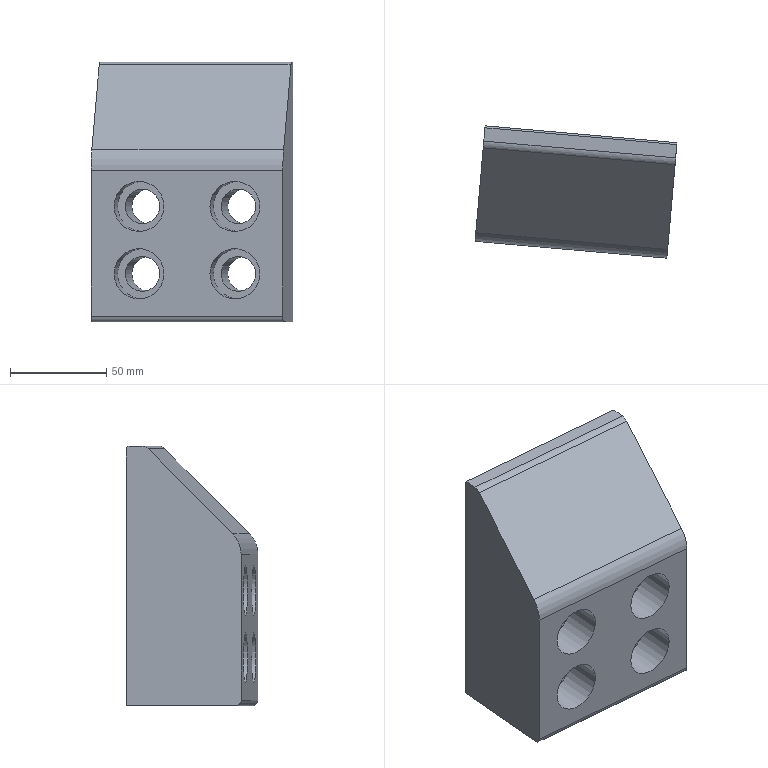Part | NX | features solid 2 | 1 solid | 23 faces | box 104.849 x 68.487 x 135 mm | volume 601030 mm3 | plane 12 | cylinder 11 | commonest cylinder face diameters 18 x4 26 x4 6 x1 10 x1 30 x1
STEP:
#1=CARTESIAN_POINT('',(231.007,-228.001,-65.));
#2=VERTEX_POINT('',#1);
#3=CARTESIAN_POINT('',(235.975,-171.218,-65.));
#4=VERTEX_POINT('',#3);
#5=CARTESIAN_POINT('',(229.874,-240.952,-65.));
#6=DIRECTION('',(0.08716,0.9962,0.));
#7=VECTOR('',#6,1000.);
#8=LINE('',#5,#7);
#9=EDGE_CURVE('',#2,#4,#8,.T.);
#10=ORIENTED_EDGE('',*,*,#9,.F.);
#11=CARTESIAN_POINT('',(230.746,-230.99,-62.));
#12=VERTEX_POINT('',#11);
#13=CARTESIAN_POINT('',(231.007,-228.001,-62.));
#14=DIRECTION('',(0.9962,-0.08716,0.));
#15=DIRECTION('',(0.,0.,1.));
#16=AXIS2_PLACEMENT_3D('',#13,#14,#15);
#17=CIRCLE('',#16,3.);
#18=EDGE_CURVE('',#2,#12,#17,.F.);
#19=ORIENTED_EDGE('',*,*,#18,.T.);
#20=CARTESIAN_POINT('',(230.746,-230.99,13.787));
#21=VERTEX_POINT('',#20);
#22=CARTESIAN_POINT('',(230.746,-230.99,-100.));
#23=DIRECTION('',(0.,0.,-1.));
#24=VECTOR('',#23,1000.);
#25=LINE('',#22,#24);
#26=EDGE_CURVE('',#21,#12,#25,.T.);
#27=ORIENTED_EDGE('',*,*,#26,.F.);
#28=CARTESIAN_POINT('',(231.129,-226.613,24.393));
#29=VERTEX_POINT('',#28);
#30=CARTESIAN_POINT('',(232.053,-216.047,13.787));
#31=DIRECTION('',(0.9962,-0.08716,0.));
#32=DIRECTION('',(0.,0.,1.));
#33=AXIS2_PLACEMENT_3D('',#30,#31,#32);
#34=CIRCLE('',#33,15.);
#35=EDGE_CURVE('',#21,#29,#34,.F.);
#36=ORIENTED_EDGE('',*,*,#35,.T.);
#37=CARTESIAN_POINT('',(234.976,-182.639,68.536));
#38=VERTEX_POINT('',#37);
#39=CARTESIAN_POINT('',(232.489,-211.066,40.));
#40=DIRECTION('',(0.06163,0.7044,0.7071));
#41=VECTOR('',#40,1000.);
#42=LINE('',#39,#41);
#43=EDGE_CURVE('',#29,#38,#42,.T.);
#44=ORIENTED_EDGE('',*,*,#43,.T.);
#45=CARTESIAN_POINT('',(235.284,-179.117,70.));
#46=VERTEX_POINT('',#45);
#47=CARTESIAN_POINT('',(235.284,-179.117,65.));
#48=DIRECTION('',(0.9962,-0.08716,0.));
#49=DIRECTION('',(0.,0.,1.));
#50=AXIS2_PLACEMENT_3D('',#47,#48,#49);
#51=CIRCLE('',#50,5.);
#52=EDGE_CURVE('',#38,#46,#51,.F.);
#53=ORIENTED_EDGE('',*,*,#52,.T.);
#54=CARTESIAN_POINT('',(235.888,-172.214,70.));
#55=VERTEX_POINT('',#54);
#56=CARTESIAN_POINT('',(229.874,-240.952,70.));
#57=DIRECTION('',(0.08716,0.9962,0.));
#58=VECTOR('',#57,1000.);
#59=LINE('',#56,#58);
#60=EDGE_CURVE('',#46,#55,#59,.T.);
#61=ORIENTED_EDGE('',*,*,#60,.T.);
#62=CARTESIAN_POINT('',(235.975,-171.218,69.));
#63=VERTEX_POINT('',#62);
#64=CARTESIAN_POINT('',(235.888,-172.214,70.));
#65=DIRECTION('',(0.06163,0.7044,-0.7071));
#66=VECTOR('',#65,1000.);
#67=LINE('',#64,#66);
#68=EDGE_CURVE('',#55,#63,#67,.T.);
#69=ORIENTED_EDGE('',*,*,#68,.T.);
#70=CARTESIAN_POINT('',(235.975,-171.218,70.));
#71=DIRECTION('',(0.,0.,-1.));
#72=VECTOR('',#71,1000.);
#73=LINE('',#70,#72);
#74=EDGE_CURVE('',#63,#4,#73,.T.);
#75=ORIENTED_EDGE('',*,*,#74,.T.);
#76=EDGE_LOOP('',(#10,#19,#27,#36,#44,#53,#61,#69,#75));
#77=FACE_BOUND('',#76,.T.);
#78=CARTESIAN_POINT('',(229.874,-240.952,70.));
#79=DIRECTION('',(0.9962,-0.08716,0.));
#80=DIRECTION('',(0.,0.,1.));
#81=AXIS2_PLACEMENT_3D('',#78,#79,#80);
#82=PLANE('',#81);
#83=ADVANCED_FACE('',(#77),#82,.F.);
#84=CARTESIAN_POINT('',(330.627,-236.717,-65.));
#85=VERTEX_POINT('',#84);
#86=CARTESIAN_POINT('',(335.595,-179.934,-65.));
#87=VERTEX_POINT('',#86);
#88=CARTESIAN_POINT('',(329.494,-249.667,-65.));
#89=DIRECTION('',(0.08716,0.9962,0.));
#90=VECTOR('',#89,1000.);
#91=LINE('',#88,#90);
#92=EDGE_CURVE('',#85,#87,#91,.T.);
#93=ORIENTED_EDGE('',*,*,#92,.F.);
#94=CARTESIAN_POINT('',(231.007,-228.001,-65.));
#95=DIRECTION('',(-0.9962,0.08716,0.));
#96=VECTOR('',#95,1000.);
#97=LINE('',#94,#96);
#98=EDGE_CURVE('',#85,#2,#97,.T.);
#99=ORIENTED_EDGE('',*,*,#98,.T.);
#100=ORIENTED_EDGE('',*,*,#9,.T.);
#101=CARTESIAN_POINT('',(335.595,-179.934,-65.));
#102=DIRECTION('',(-0.9962,0.08716,0.));
#103=VECTOR('',#102,1000.);
#104=LINE('',#101,#103);
#105=EDGE_CURVE('',#87,#4,#104,.T.);
#106=ORIENTED_EDGE('',*,*,#105,.F.);
#107=EDGE_LOOP('',(#93,#99,#100,#106));
#108=FACE_BOUND('',#107,.T.);
#109=CARTESIAN_POINT('',(329.494,-249.667,-65.));
#110=DIRECTION('',(0.,0.,-1.));
#111=DIRECTION('',(0.08716,0.9962,0.));
#112=AXIS2_PLACEMENT_3D('',#109,#110,#111);
#113=PLANE('',#112);
#114=ADVANCED_FACE('',(#108),#113,.T.);
#115=CARTESIAN_POINT('',(330.365,-239.705,13.787));
#116=VERTEX_POINT('',#115);
#117=CARTESIAN_POINT('',(330.365,-239.705,-62.));
#118=VERTEX_POINT('',#117);
#119=CARTESIAN_POINT('',(330.365,-239.705,-100.));
#120=DIRECTION('',(0.,0.,-1.));
#121=VECTOR('',#120,1000.);
#122=LINE('',#119,#121);
#123=EDGE_CURVE('',#116,#118,#122,.T.);
#124=ORIENTED_EDGE('',*,*,#123,.T.);
#125=CARTESIAN_POINT('',(330.627,-236.717,-62.));
#126=DIRECTION('',(0.9962,-0.08716,0.));
#127=DIRECTION('',(0.,0.,1.));
#128=AXIS2_PLACEMENT_3D('',#125,#126,#127);
#129=CIRCLE('',#128,3.);
#130=EDGE_CURVE('',#118,#85,#129,.T.);
#131=ORIENTED_EDGE('',*,*,#130,.T.);
#132=ORIENTED_EDGE('',*,*,#92,.T.);
#133=CARTESIAN_POINT('',(335.595,-179.934,69.));
#134=VERTEX_POINT('',#133);
#135=CARTESIAN_POINT('',(335.595,-179.934,70.));
#136=DIRECTION('',(0.,0.,-1.));
#137=VECTOR('',#136,1000.);
#138=LINE('',#135,#137);
#139=EDGE_CURVE('',#134,#87,#138,.T.);
#140=ORIENTED_EDGE('',*,*,#139,.F.);
#141=CARTESIAN_POINT('',(335.508,-180.93,70.));
#142=VERTEX_POINT('',#141);
#143=CARTESIAN_POINT('',(332.501,-215.299,104.5));
#144=DIRECTION('',(-0.06163,-0.7044,0.7071));
#145=VECTOR('',#144,1000.);
#146=LINE('',#143,#145);
#147=EDGE_CURVE('',#134,#142,#146,.T.);
#148=ORIENTED_EDGE('',*,*,#147,.T.);
#149=CARTESIAN_POINT('',(334.904,-187.832,70.));
#150=VERTEX_POINT('',#149);
#151=CARTESIAN_POINT('',(329.494,-249.667,70.));
#152=DIRECTION('',(0.08716,0.9962,0.));
#153=VECTOR('',#152,1000.);
#154=LINE('',#151,#153);
#155=EDGE_CURVE('',#150,#142,#154,.T.);
#156=ORIENTED_EDGE('',*,*,#155,.F.);
#157=CARTESIAN_POINT('',(334.596,-191.355,68.536));
#158=VERTEX_POINT('',#157);
#159=CARTESIAN_POINT('',(334.904,-187.832,65.));
#160=DIRECTION('',(0.9962,-0.08716,0.));
#161=DIRECTION('',(0.,0.,1.));
#162=AXIS2_PLACEMENT_3D('',#159,#160,#161);
#163=CIRCLE('',#162,5.);
#164=EDGE_CURVE('',#150,#158,#163,.T.);
#165=ORIENTED_EDGE('',*,*,#164,.T.);
#166=CARTESIAN_POINT('',(330.748,-235.329,24.393));
#167=VERTEX_POINT('',#166);
#168=CARTESIAN_POINT('',(332.109,-219.782,40.));
#169=DIRECTION('',(0.06163,0.7044,0.7071));
#170=VECTOR('',#169,1000.);
#171=LINE('',#168,#170);
#172=EDGE_CURVE('',#167,#158,#171,.T.);
#173=ORIENTED_EDGE('',*,*,#172,.F.);
#174=CARTESIAN_POINT('',(331.673,-224.762,13.787));
#175=DIRECTION('',(0.9962,-0.08716,0.));
#176=DIRECTION('',(0.,0.,1.));
#177=AXIS2_PLACEMENT_3D('',#174,#175,#176);
#178=CIRCLE('',#177,15.);
#179=EDGE_CURVE('',#167,#116,#178,.T.);
#180=ORIENTED_EDGE('',*,*,#179,.T.);
#181=EDGE_LOOP('',(#124,#131,#132,#140,#148,#156,#165,#173,#180));
#182=FACE_BOUND('',#181,.T.);
#183=CARTESIAN_POINT('',(329.494,-249.667,70.));
#184=DIRECTION('',(0.9962,-0.08716,0.));
#185=DIRECTION('',(0.,0.,1.));
#186=AXIS2_PLACEMENT_3D('',#183,#184,#185);
#187=PLANE('',#186);
#188=ADVANCED_FACE('',(#182),#187,.T.);
#189=ORIENTED_EDGE('',*,*,#155,.T.);
#190=CARTESIAN_POINT('',(235.888,-172.214,70.));
#191=DIRECTION('',(-0.9962,0.08716,0.));
#192=VECTOR('',#191,1000.);
#193=LINE('',#190,#192);
#194=EDGE_CURVE('',#142,#55,#193,.T.);
#195=ORIENTED_EDGE('',*,*,#194,.T.);
#196=ORIENTED_EDGE('',*,*,#60,.F.);
#197=CARTESIAN_POINT('',(334.904,-187.832,70.));
#198=DIRECTION('',(0.9962,-0.08716,0.));
#199=VECTOR('',#198,1000.);
#200=LINE('',#197,#199);
#201=EDGE_CURVE('',#46,#150,#200,.T.);
#202=ORIENTED_EDGE('',*,*,#201,.T.);
#203=EDGE_LOOP('',(#189,#195,#196,#202));
#204=FACE_BOUND('',#203,.T.);
#205=CARTESIAN_POINT('',(329.494,-249.667,70.));
#206=DIRECTION('',(0.,0.,-1.));
#207=DIRECTION('',(0.08716,0.9962,0.));
#208=AXIS2_PLACEMENT_3D('',#205,#206,#207);
#209=PLANE('',#208);
#210=ADVANCED_FACE('',(#204),#209,.F.);
#211=CARTESIAN_POINT('',(242.7,-232.036,-40.));
#212=VERTEX_POINT('',#211);
#213=CARTESIAN_POINT('',(255.651,-233.169,-40.));
#214=DIRECTION('',(0.08716,0.9962,0.));
#215=DIRECTION('',(-0.9962,0.08716,0.));
#216=AXIS2_PLACEMENT_3D('',#213,#214,#215);
#217=CIRCLE('',#216,13.);
#218=EDGE_CURVE('',#212,#212,#217,.T.);
#219=ORIENTED_EDGE('',*,*,#218,.T.);
#220=EDGE_LOOP('',(#219));
#221=FACE_BOUND('',#220,.T.);
#222=CARTESIAN_POINT('',(292.51,-236.393,-40.));
#223=VERTEX_POINT('',#222);
#224=CARTESIAN_POINT('',(305.461,-237.527,-40.));
#225=DIRECTION('',(0.08716,0.9962,0.));
#226=DIRECTION('',(-0.9962,0.08716,0.));
#227=AXIS2_PLACEMENT_3D('',#224,#225,#226);
#228=CIRCLE('',#227,13.);
#229=EDGE_CURVE('',#223,#223,#228,.T.);
#230=ORIENTED_EDGE('',*,*,#229,.T.);
#231=EDGE_LOOP('',(#230));
#232=FACE_BOUND('',#231,.T.);
#233=CARTESIAN_POINT('',(292.51,-236.393,-5.));
#234=VERTEX_POINT('',#233);
#235=CARTESIAN_POINT('',(305.461,-237.527,-5.));
#236=DIRECTION('',(0.08716,0.9962,0.));
#237=DIRECTION('',(-0.9962,0.08716,0.));
#238=AXIS2_PLACEMENT_3D('',#235,#236,#237);
#239=CIRCLE('',#238,13.);
#240=EDGE_CURVE('',#234,#234,#239,.T.);
#241=ORIENTED_EDGE('',*,*,#240,.T.);
#242=EDGE_LOOP('',(#241));
#243=FACE_BOUND('',#242,.T.);
#244=CARTESIAN_POINT('',(242.7,-232.036,-5.));
#245=VERTEX_POINT('',#244);
#246=CARTESIAN_POINT('',(255.651,-233.169,-5.));
#247=DIRECTION('',(0.08716,0.9962,0.));
#248=DIRECTION('',(-0.9962,0.08716,0.));
#249=AXIS2_PLACEMENT_3D('',#246,#247,#248);
#250=CIRCLE('',#249,13.);
#251=EDGE_CURVE('',#245,#245,#250,.T.);
#252=ORIENTED_EDGE('',*,*,#251,.T.);
#253=EDGE_LOOP('',(#252));
#254=FACE_BOUND('',#253,.T.);
#255=ORIENTED_EDGE('',*,*,#26,.T.);
#256=CARTESIAN_POINT('',(330.365,-239.705,-62.));
#257=DIRECTION('',(-0.9962,0.08716,0.));
#258=VECTOR('',#257,1000.);
#259=LINE('',#256,#258);
#260=EDGE_CURVE('',#12,#118,#259,.F.);
#261=ORIENTED_EDGE('',*,*,#260,.T.);
#262=ORIENTED_EDGE('',*,*,#123,.F.);
#263=CARTESIAN_POINT('',(230.746,-230.99,13.787));
#264=DIRECTION('',(-0.9962,0.08716,0.));
#265=VECTOR('',#264,1000.);
#266=LINE('',#263,#265);
#267=EDGE_CURVE('',#116,#21,#266,.T.);
#268=ORIENTED_EDGE('',*,*,#267,.T.);
#269=EDGE_LOOP('',(#255,#261,#262,#268));
#270=FACE_BOUND('',#269,.T.);
#271=CARTESIAN_POINT('',(230.746,-230.99,-100.));
#272=DIRECTION('',(0.08716,0.9962,0.));
#273=DIRECTION('',(-0.9962,0.08716,0.));
#274=AXIS2_PLACEMENT_3D('',#271,#272,#273);
#275=PLANE('',#274);
#276=ADVANCED_FACE('',(#221,#232,#243,#254,#270),#275,.F.);
#277=CARTESIAN_POINT('',(251.914,-172.613,-40.));
#278=VERTEX_POINT('',#277);
#279=CARTESIAN_POINT('',(260.88,-173.397,-40.));
#280=DIRECTION('',(0.08716,0.9962,0.));
#281=DIRECTION('',(-0.9962,0.08716,0.));
#282=AXIS2_PLACEMENT_3D('',#279,#280,#281);
#283=CIRCLE('',#282,9.);
#284=EDGE_CURVE('',#278,#278,#283,.T.);
#285=ORIENTED_EDGE('',*,*,#284,.F.);
#286=EDGE_LOOP('',(#285));
#287=FACE_BOUND('',#286,.T.);
#288=CARTESIAN_POINT('',(301.724,-176.97,-40.));
#289=VERTEX_POINT('',#288);
#290=CARTESIAN_POINT('',(310.69,-177.755,-40.));
#291=DIRECTION('',(0.08716,0.9962,0.));
#292=DIRECTION('',(-0.9962,0.08716,0.));
#293=AXIS2_PLACEMENT_3D('',#290,#291,#292);
#294=CIRCLE('',#293,9.);
#295=EDGE_CURVE('',#289,#289,#294,.T.);
#296=ORIENTED_EDGE('',*,*,#295,.F.);
#297=EDGE_LOOP('',(#296));
#298=FACE_BOUND('',#297,.T.);
#299=CARTESIAN_POINT('',(301.724,-176.97,-5.));
#300=VERTEX_POINT('',#299);
#301=CARTESIAN_POINT('',(310.69,-177.755,-5.));
#302=DIRECTION('',(0.08716,0.9962,0.));
#303=DIRECTION('',(-0.9962,0.08716,0.));
#304=AXIS2_PLACEMENT_3D('',#301,#302,#303);
#305=CIRCLE('',#304,9.);
#306=EDGE_CURVE('',#300,#300,#305,.T.);
#307=ORIENTED_EDGE('',*,*,#306,.F.);
#308=EDGE_LOOP('',(#307));
#309=FACE_BOUND('',#308,.T.);
#310=CARTESIAN_POINT('',(251.914,-172.613,-5.));
#311=VERTEX_POINT('',#310);
#312=CARTESIAN_POINT('',(260.88,-173.397,-5.));
#313=DIRECTION('',(0.08716,0.9962,0.));
#314=DIRECTION('',(-0.9962,0.08716,0.));
#315=AXIS2_PLACEMENT_3D('',#312,#313,#314);
#316=CIRCLE('',#315,9.);
#317=EDGE_CURVE('',#311,#311,#316,.T.);
#318=ORIENTED_EDGE('',*,*,#317,.F.);
#319=EDGE_LOOP('',(#318));
#320=FACE_BOUND('',#319,.T.);
#321=ORIENTED_EDGE('',*,*,#74,.F.);
#322=CARTESIAN_POINT('',(335.595,-179.934,69.));
#323=DIRECTION('',(0.9962,-0.08716,0.));
#324=VECTOR('',#323,1000.);
#325=LINE('',#322,#324);
#326=EDGE_CURVE('',#63,#134,#325,.T.);
#327=ORIENTED_EDGE('',*,*,#326,.T.);
#328=ORIENTED_EDGE('',*,*,#139,.T.);
#329=ORIENTED_EDGE('',*,*,#105,.T.);
#330=EDGE_LOOP('',(#321,#327,#328,#329));
#331=FACE_BOUND('',#330,.T.);
#332=CARTESIAN_POINT('',(235.975,-171.218,-100.));
#333=DIRECTION('',(0.08716,0.9962,0.));
#334=DIRECTION('',(-0.9962,0.08716,0.));
#335=AXIS2_PLACEMENT_3D('',#332,#333,#334);
#336=PLANE('',#335);
#337=ADVANCED_FACE('',(#287,#298,#309,#320,#331),#336,.T.);
#338=ORIENTED_EDGE('',*,*,#43,.F.);
#339=CARTESIAN_POINT('',(231.129,-226.613,24.393));
#340=DIRECTION('',(-0.9962,0.08716,0.));
#341=VECTOR('',#340,1000.);
#342=LINE('',#339,#341);
#343=EDGE_CURVE('',#29,#167,#342,.F.);
#344=ORIENTED_EDGE('',*,*,#343,.T.);
#345=ORIENTED_EDGE('',*,*,#172,.T.);
#346=CARTESIAN_POINT('',(234.976,-182.639,68.536));
#347=DIRECTION('',(0.9962,-0.08716,0.));
#348=VECTOR('',#347,1000.);
#349=LINE('',#346,#348);
#350=EDGE_CURVE('',#158,#38,#349,.F.);
#351=ORIENTED_EDGE('',*,*,#350,.T.);
#352=EDGE_LOOP('',(#338,#344,#345,#351));
#353=FACE_BOUND('',#352,.T.);
#354=CARTESIAN_POINT('',(224.627,-300.931,-50.208));
#355=DIRECTION('',(0.06163,0.7044,-0.7071));
#356=DIRECTION('',(0.06163,0.7044,0.7071));
#357=AXIS2_PLACEMENT_3D('',#354,#355,#356);
#358=PLANE('',#357);
#359=ADVANCED_FACE('',(#353),#358,.F.);
#360=CARTESIAN_POINT('',(270.344,-214.378,-5.));
#361=VERTEX_POINT('',#360);
#362=CARTESIAN_POINT('',(257.394,-213.245,-5.));
#363=DIRECTION('',(-0.08716,-0.9962,0.));
#364=DIRECTION('',(0.9962,-0.08716,0.));
#365=AXIS2_PLACEMENT_3D('',#362,#363,#364);
#366=CIRCLE('',#365,13.);
#367=EDGE_CURVE('',#361,#361,#366,.T.);
#368=ORIENTED_EDGE('',*,*,#367,.F.);
#369=EDGE_LOOP('',(#368));
#370=FACE_BOUND('',#369,.T.);
#371=ORIENTED_EDGE('',*,*,#251,.F.);
#372=EDGE_LOOP('',(#371));
#373=FACE_BOUND('',#372,.T.);
#374=CARTESIAN_POINT('',(257.394,-213.245,-5.));
#375=DIRECTION('',(-0.08716,-0.9962,0.));
#376=DIRECTION('',(0.9962,-0.08716,0.));
#377=AXIS2_PLACEMENT_3D('',#374,#375,#376);
#378=CYLINDRICAL_SURFACE('',#377,13.);
#379=ADVANCED_FACE('',(#370,#373),#378,.F.);
#380=ORIENTED_EDGE('',*,*,#317,.T.);
#381=EDGE_LOOP('',(#380));
#382=FACE_BOUND('',#381,.T.);
#383=CARTESIAN_POINT('',(248.428,-212.46,-5.));
#384=VERTEX_POINT('',#383);
#385=CARTESIAN_POINT('',(257.394,-213.245,-5.));
#386=DIRECTION('',(0.08716,0.9962,0.));
#387=DIRECTION('',(-0.9962,0.08716,0.));
#388=AXIS2_PLACEMENT_3D('',#385,#386,#387);
#389=CIRCLE('',#388,9.);
#390=EDGE_CURVE('',#384,#384,#389,.F.);
#391=ORIENTED_EDGE('',*,*,#390,.T.);
#392=EDGE_LOOP('',(#391));
#393=FACE_BOUND('',#392,.T.);
#394=CARTESIAN_POINT('',(264.366,-133.549,-5.));
#395=DIRECTION('',(-0.08716,-0.9962,0.));
#396=DIRECTION('',(0.9962,-0.08716,0.));
#397=AXIS2_PLACEMENT_3D('',#394,#395,#396);
#398=CYLINDRICAL_SURFACE('',#397,9.);
#399=ADVANCED_FACE('',(#382,#393),#398,.F.);
#400=ORIENTED_EDGE('',*,*,#390,.F.);
#401=EDGE_LOOP('',(#400));
#402=FACE_BOUND('',#401,.T.);
#403=ORIENTED_EDGE('',*,*,#367,.T.);
#404=EDGE_LOOP('',(#403));
#405=FACE_BOUND('',#404,.T.);
#406=CARTESIAN_POINT('',(257.394,-213.245,-5.));
#407=DIRECTION('',(0.08716,0.9962,0.));
#408=DIRECTION('',(-0.9962,0.08716,0.));
#409=AXIS2_PLACEMENT_3D('',#406,#407,#408);
#410=PLANE('',#409);
#411=ADVANCED_FACE('',(#402,#405),#410,.F.);
#412=CARTESIAN_POINT('',(320.154,-218.736,-5.));
#413=VERTEX_POINT('',#412);
#414=CARTESIAN_POINT('',(307.204,-217.603,-5.));
#415=DIRECTION('',(-0.08716,-0.9962,0.));
#416=DIRECTION('',(0.9962,-0.08716,0.));
#417=AXIS2_PLACEMENT_3D('',#414,#415,#416);
#418=CIRCLE('',#417,13.);
#419=EDGE_CURVE('',#413,#413,#418,.T.);
#420=ORIENTED_EDGE('',*,*,#419,.F.);
#421=EDGE_LOOP('',(#420));
#422=FACE_BOUND('',#421,.T.);
#423=ORIENTED_EDGE('',*,*,#240,.F.);
#424=EDGE_LOOP('',(#423));
#425=FACE_BOUND('',#424,.T.);
#426=CARTESIAN_POINT('',(307.204,-217.603,-5.));
#427=DIRECTION('',(-0.08716,-0.9962,0.));
#428=DIRECTION('',(0.9962,-0.08716,0.));
#429=AXIS2_PLACEMENT_3D('',#426,#427,#428);
#430=CYLINDRICAL_SURFACE('',#429,13.);
#431=ADVANCED_FACE('',(#422,#425),#430,.F.);
#432=ORIENTED_EDGE('',*,*,#306,.T.);
#433=EDGE_LOOP('',(#432));
#434=FACE_BOUND('',#433,.T.);
#435=CARTESIAN_POINT('',(298.238,-216.818,-5.));
#436=VERTEX_POINT('',#435);
#437=CARTESIAN_POINT('',(307.204,-217.603,-5.));
#438=DIRECTION('',(0.08716,0.9962,0.));
#439=DIRECTION('',(-0.9962,0.08716,0.));
#440=AXIS2_PLACEMENT_3D('',#437,#438,#439);
#441=CIRCLE('',#440,9.);
#442=EDGE_CURVE('',#436,#436,#441,.F.);
#443=ORIENTED_EDGE('',*,*,#442,.T.);
#444=EDGE_LOOP('',(#443));
#445=FACE_BOUND('',#444,.T.);
#446=CARTESIAN_POINT('',(314.176,-137.907,-5.));
#447=DIRECTION('',(-0.08716,-0.9962,0.));
#448=DIRECTION('',(0.9962,-0.08716,0.));
#449=AXIS2_PLACEMENT_3D('',#446,#447,#448);
#450=CYLINDRICAL_SURFACE('',#449,9.);
#451=ADVANCED_FACE('',(#434,#445),#450,.F.);
#452=ORIENTED_EDGE('',*,*,#442,.F.);
#453=EDGE_LOOP('',(#452));
#454=FACE_BOUND('',#453,.T.);
#455=ORIENTED_EDGE('',*,*,#419,.T.);
#456=EDGE_LOOP('',(#455));
#457=FACE_BOUND('',#456,.T.);
#458=CARTESIAN_POINT('',(307.204,-217.603,-5.));
#459=DIRECTION('',(0.08716,0.9962,0.));
#460=DIRECTION('',(-0.9962,0.08716,0.));
#461=AXIS2_PLACEMENT_3D('',#458,#459,#460);
#462=PLANE('',#461);
#463=ADVANCED_FACE('',(#454,#457),#462,.F.);
#464=CARTESIAN_POINT('',(320.154,-218.736,-40.));
#465=VERTEX_POINT('',#464);
#466=CARTESIAN_POINT('',(307.204,-217.603,-40.));
#467=DIRECTION('',(-0.08716,-0.9962,0.));
#468=DIRECTION('',(0.9962,-0.08716,0.));
#469=AXIS2_PLACEMENT_3D('',#466,#467,#468);
#470=CIRCLE('',#469,13.);
#471=EDGE_CURVE('',#465,#465,#470,.T.);
#472=ORIENTED_EDGE('',*,*,#471,.F.);
#473=EDGE_LOOP('',(#472));
#474=FACE_BOUND('',#473,.T.);
#475=ORIENTED_EDGE('',*,*,#229,.F.);
#476=EDGE_LOOP('',(#475));
#477=FACE_BOUND('',#476,.T.);
#478=CARTESIAN_POINT('',(307.204,-217.603,-40.));
#479=DIRECTION('',(-0.08716,-0.9962,0.));
#480=DIRECTION('',(0.9962,-0.08716,0.));
#481=AXIS2_PLACEMENT_3D('',#478,#479,#480);
#482=CYLINDRICAL_SURFACE('',#481,13.);
#483=ADVANCED_FACE('',(#474,#477),#482,.F.);
#484=ORIENTED_EDGE('',*,*,#295,.T.);
#485=EDGE_LOOP('',(#484));
#486=FACE_BOUND('',#485,.T.);
#487=CARTESIAN_POINT('',(298.238,-216.818,-40.));
#488=VERTEX_POINT('',#487);
#489=CARTESIAN_POINT('',(307.204,-217.603,-40.));
#490=DIRECTION('',(0.08716,0.9962,0.));
#491=DIRECTION('',(-0.9962,0.08716,0.));
#492=AXIS2_PLACEMENT_3D('',#489,#490,#491);
#493=CIRCLE('',#492,9.);
#494=EDGE_CURVE('',#488,#488,#493,.F.);
#495=ORIENTED_EDGE('',*,*,#494,.T.);
#496=EDGE_LOOP('',(#495));
#497=FACE_BOUND('',#496,.T.);
#498=CARTESIAN_POINT('',(314.176,-137.907,-40.));
#499=DIRECTION('',(-0.08716,-0.9962,0.));
#500=DIRECTION('',(0.9962,-0.08716,0.));
#501=AXIS2_PLACEMENT_3D('',#498,#499,#500);
#502=CYLINDRICAL_SURFACE('',#501,9.);
#503=ADVANCED_FACE('',(#486,#497),#502,.F.);
#504=ORIENTED_EDGE('',*,*,#494,.F.);
#505=EDGE_LOOP('',(#504));
#506=FACE_BOUND('',#505,.T.);
#507=ORIENTED_EDGE('',*,*,#471,.T.);
#508=EDGE_LOOP('',(#507));
#509=FACE_BOUND('',#508,.T.);
#510=CARTESIAN_POINT('',(307.204,-217.603,-40.));
#511=DIRECTION('',(0.08716,0.9962,0.));
#512=DIRECTION('',(-0.9962,0.08716,0.));
#513=AXIS2_PLACEMENT_3D('',#510,#511,#512);
#514=PLANE('',#513);
#515=ADVANCED_FACE('',(#506,#509),#514,.F.);
#516=CARTESIAN_POINT('',(270.344,-214.378,-40.));
#517=VERTEX_POINT('',#516);
#518=CARTESIAN_POINT('',(257.394,-213.245,-40.));
#519=DIRECTION('',(-0.08716,-0.9962,0.));
#520=DIRECTION('',(0.9962,-0.08716,0.));
#521=AXIS2_PLACEMENT_3D('',#518,#519,#520);
#522=CIRCLE('',#521,13.);
#523=EDGE_CURVE('',#517,#517,#522,.T.);
#524=ORIENTED_EDGE('',*,*,#523,.F.);
#525=EDGE_LOOP('',(#524));
#526=FACE_BOUND('',#525,.T.);
#527=ORIENTED_EDGE('',*,*,#218,.F.);
#528=EDGE_LOOP('',(#527));
#529=FACE_BOUND('',#528,.T.);
#530=CARTESIAN_POINT('',(257.394,-213.245,-40.));
#531=DIRECTION('',(-0.08716,-0.9962,0.));
#532=DIRECTION('',(0.9962,-0.08716,0.));
#533=AXIS2_PLACEMENT_3D('',#530,#531,#532);
#534=CYLINDRICAL_SURFACE('',#533,13.);
#535=ADVANCED_FACE('',(#526,#529),#534,.F.);
#536=ORIENTED_EDGE('',*,*,#284,.T.);
#537=EDGE_LOOP('',(#536));
#538=FACE_BOUND('',#537,.T.);
#539=CARTESIAN_POINT('',(248.428,-212.46,-40.));
#540=VERTEX_POINT('',#539);
#541=CARTESIAN_POINT('',(257.394,-213.245,-40.));
#542=DIRECTION('',(0.08716,0.9962,0.));
#543=DIRECTION('',(-0.9962,0.08716,0.));
#544=AXIS2_PLACEMENT_3D('',#541,#542,#543);
#545=CIRCLE('',#544,9.);
#546=EDGE_CURVE('',#540,#540,#545,.F.);
#547=ORIENTED_EDGE('',*,*,#546,.T.);
#548=EDGE_LOOP('',(#547));
#549=FACE_BOUND('',#548,.T.);
#550=CARTESIAN_POINT('',(264.366,-133.549,-40.));
#551=DIRECTION('',(-0.08716,-0.9962,0.));
#552=DIRECTION('',(0.9962,-0.08716,0.));
#553=AXIS2_PLACEMENT_3D('',#550,#551,#552);
#554=CYLINDRICAL_SURFACE('',#553,9.);
#555=ADVANCED_FACE('',(#538,#549),#554,.F.);
#556=ORIENTED_EDGE('',*,*,#546,.F.);
#557=EDGE_LOOP('',(#556));
#558=FACE_BOUND('',#557,.T.);
#559=ORIENTED_EDGE('',*,*,#523,.T.);
#560=EDGE_LOOP('',(#559));
#561=FACE_BOUND('',#560,.T.);
#562=CARTESIAN_POINT('',(257.394,-213.245,-40.));
#563=DIRECTION('',(0.08716,0.9962,0.));
#564=DIRECTION('',(-0.9962,0.08716,0.));
#565=AXIS2_PLACEMENT_3D('',#562,#563,#564);
#566=PLANE('',#565);
#567=ADVANCED_FACE('',(#558,#561),#566,.F.);
#568=ORIENTED_EDGE('',*,*,#52,.F.);
#569=ORIENTED_EDGE('',*,*,#350,.F.);
#570=ORIENTED_EDGE('',*,*,#164,.F.);
#571=ORIENTED_EDGE('',*,*,#201,.F.);
#572=EDGE_LOOP('',(#568,#569,#570,#571));
#573=FACE_BOUND('',#572,.T.);
#574=CARTESIAN_POINT('',(334.904,-187.832,65.));
#575=DIRECTION('',(0.9962,-0.08716,0.));
#576=DIRECTION('',(0.08716,0.9962,0.));
#577=AXIS2_PLACEMENT_3D('',#574,#575,#576);
#578=CYLINDRICAL_SURFACE('',#577,5.);
#579=ADVANCED_FACE('',(#573),#578,.T.);
#580=ORIENTED_EDGE('',*,*,#179,.F.);
#581=ORIENTED_EDGE('',*,*,#343,.F.);
#582=ORIENTED_EDGE('',*,*,#35,.F.);
#583=ORIENTED_EDGE('',*,*,#267,.F.);
#584=EDGE_LOOP('',(#580,#581,#582,#583));
#585=FACE_BOUND('',#584,.T.);
#586=CARTESIAN_POINT('',(232.053,-216.047,13.787));
#587=DIRECTION('',(-0.9962,0.08716,0.));
#588=DIRECTION('',(-0.08716,-0.9962,0.));
#589=AXIS2_PLACEMENT_3D('',#586,#587,#588);
#590=CYLINDRICAL_SURFACE('',#589,15.);
#591=ADVANCED_FACE('',(#585),#590,.T.);
#592=ORIENTED_EDGE('',*,*,#147,.F.);
#593=ORIENTED_EDGE('',*,*,#326,.F.);
#594=ORIENTED_EDGE('',*,*,#68,.F.);
#595=ORIENTED_EDGE('',*,*,#194,.F.);
#596=EDGE_LOOP('',(#592,#593,#594,#595));
#597=FACE_BOUND('',#596,.T.);
#598=CARTESIAN_POINT('',(335.508,-180.93,70.));
#599=DIRECTION('',(0.06163,0.7044,0.7071));
#600=DIRECTION('',(-0.06163,-0.7044,0.7071));
#601=AXIS2_PLACEMENT_3D('',#598,#599,#600);
#602=PLANE('',#601);
#603=ADVANCED_FACE('',(#597),#602,.T.);
#604=ORIENTED_EDGE('',*,*,#130,.F.);
#605=ORIENTED_EDGE('',*,*,#260,.F.);
#606=ORIENTED_EDGE('',*,*,#18,.F.);
#607=ORIENTED_EDGE('',*,*,#98,.F.);
#608=EDGE_LOOP('',(#604,#605,#606,#607));
#609=FACE_BOUND('',#608,.T.);
#610=CARTESIAN_POINT('',(330.627,-236.717,-62.));
#611=DIRECTION('',(0.9962,-0.08716,0.));
#612=DIRECTION('',(0.08716,0.9962,0.));
#613=AXIS2_PLACEMENT_3D('',#610,#611,#612);
#614=CYLINDRICAL_SURFACE('',#613,3.);
#615=ADVANCED_FACE('',(#609),#614,.T.);
#616=CLOSED_SHELL('',(#83,#114,#188,#210,#276,#337,#359,#379,#399,#411,#431,#451,#463,#483,#503,#515,#535,#555,#567,#579,#591,#603,#615));
#617=MANIFOLD_SOLID_BREP('',#616);
#618=(LENGTH_UNIT()NAMED_UNIT(*)SI_UNIT(.MILLI.,.METRE.));
#619=UNCERTAINTY_MEASURE_WITH_UNIT(LENGTH_MEASURE(0.00001),#618,'','');
#620=(NAMED_UNIT(*)PLANE_ANGLE_UNIT()SI_UNIT($,.RADIAN.));
#621=(NAMED_UNIT(*)SI_UNIT($,.STERADIAN.)SOLID_ANGLE_UNIT());
#622=(GEOMETRIC_REPRESENTATION_CONTEXT(3)GLOBAL_UNCERTAINTY_ASSIGNED_CONTEXT((#619))GLOBAL_UNIT_ASSIGNED_CONTEXT((#618,#620,#621))REPRESENTATION_CONTEXT('',''));
#623=ADVANCED_BREP_SHAPE_REPRESENTATION('',(#617),#622);